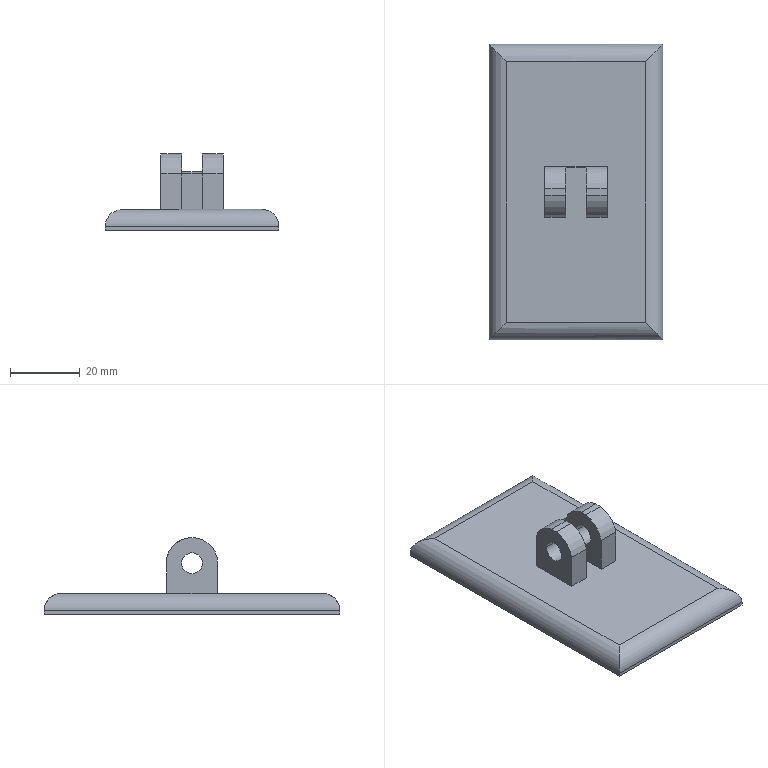Part | SolidWorks | features ICE 3, Extrusion 1, Fillet 1 | 1 solid | 27 faces | box 50 x 85 x 22 mm | volume 26297 mm3 | plane 16 | cylinder 11 | commonest cylinder face diameters 6 x4 10 x4 14.776 x3
STEP:
#1=CARTESIAN_POINT('',(34.,45.508,14.673));
#2=VERTEX_POINT('',#1);
#3=CARTESIAN_POINT('',(34.,39.508,14.673));
#4=VERTEX_POINT('',#3);
#5=CARTESIAN_POINT('',(34.,42.508,14.673));
#6=DIRECTION('',(-1.,0.,0.));
#7=DIRECTION('',(0.,-1.,0.));
#8=AXIS2_PLACEMENT_3D('',#5,#6,#7);
#9=CIRCLE('',#8,3.);
#10=EDGE_CURVE('',#2,#4,#9,.T.);
#11=ORIENTED_EDGE('',*,*,#10,.F.);
#12=CARTESIAN_POINT('',(28.,45.508,14.673));
#13=VERTEX_POINT('',#12);
#14=CARTESIAN_POINT('',(50.,45.508,14.673));
#15=DIRECTION('',(-1.,0.,0.));
#16=VECTOR('',#15,1000.);
#17=LINE('',#14,#16);
#18=EDGE_CURVE('',#2,#13,#17,.T.);
#19=ORIENTED_EDGE('',*,*,#18,.T.);
#20=CARTESIAN_POINT('',(28.,39.508,14.673));
#21=VERTEX_POINT('',#20);
#22=CARTESIAN_POINT('',(28.,42.508,14.673));
#23=DIRECTION('',(1.,0.,0.));
#24=DIRECTION('',(0.,1.,0.));
#25=AXIS2_PLACEMENT_3D('',#22,#23,#24);
#26=CIRCLE('',#25,3.);
#27=EDGE_CURVE('',#21,#13,#26,.T.);
#28=ORIENTED_EDGE('',*,*,#27,.F.);
#29=CARTESIAN_POINT('',(50.,39.508,14.673));
#30=DIRECTION('',(-1.,0.,0.));
#31=VECTOR('',#30,1000.);
#32=LINE('',#29,#31);
#33=EDGE_CURVE('',#4,#21,#32,.T.);
#34=ORIENTED_EDGE('',*,*,#33,.F.);
#35=EDGE_LOOP('',(#11,#19,#28,#34));
#36=FACE_OUTER_BOUND('',#35,.T.);
#37=CARTESIAN_POINT('',(50.,42.508,14.673));
#38=DIRECTION('',(-1.,0.,0.));
#39=DIRECTION('',(0.,-1.,0.));
#40=AXIS2_PLACEMENT_3D('',#37,#38,#39);
#41=CYLINDRICAL_SURFACE('',#40,3.);
#42=ADVANCED_FACE('',(#36),#41,.F.);
#43=CARTESIAN_POINT('',(22.,45.508,14.673));
#44=VERTEX_POINT('',#43);
#45=CARTESIAN_POINT('',(22.,39.508,14.673));
#46=VERTEX_POINT('',#45);
#47=CARTESIAN_POINT('',(22.,42.508,14.673));
#48=DIRECTION('',(-1.,0.,0.));
#49=DIRECTION('',(0.,-1.,0.));
#50=AXIS2_PLACEMENT_3D('',#47,#48,#49);
#51=CIRCLE('',#50,3.);
#52=EDGE_CURVE('',#44,#46,#51,.T.);
#53=ORIENTED_EDGE('',*,*,#52,.F.);
#54=CARTESIAN_POINT('',(16.,45.508,14.673));
#55=VERTEX_POINT('',#54);
#56=CARTESIAN_POINT('',(50.,45.508,14.673));
#57=DIRECTION('',(-1.,0.,0.));
#58=VECTOR('',#57,1000.);
#59=LINE('',#56,#58);
#60=EDGE_CURVE('',#44,#55,#59,.T.);
#61=ORIENTED_EDGE('',*,*,#60,.T.);
#62=CARTESIAN_POINT('',(16.,39.508,14.673));
#63=VERTEX_POINT('',#62);
#64=CARTESIAN_POINT('',(16.,42.508,14.673));
#65=DIRECTION('',(-1.,0.,0.));
#66=DIRECTION('',(0.,-1.,0.));
#67=AXIS2_PLACEMENT_3D('',#64,#65,#66);
#68=CIRCLE('',#67,3.);
#69=EDGE_CURVE('',#55,#63,#68,.T.);
#70=ORIENTED_EDGE('',*,*,#69,.T.);
#71=CARTESIAN_POINT('',(50.,39.508,14.673));
#72=DIRECTION('',(-1.,0.,0.));
#73=VECTOR('',#72,1000.);
#74=LINE('',#71,#73);
#75=EDGE_CURVE('',#46,#63,#74,.T.);
#76=ORIENTED_EDGE('',*,*,#75,.F.);
#77=EDGE_LOOP('',(#53,#61,#70,#76));
#78=FACE_OUTER_BOUND('',#77,.T.);
#79=CARTESIAN_POINT('',(50.,42.508,14.673));
#80=DIRECTION('',(-1.,0.,0.));
#81=DIRECTION('',(0.,-1.,0.));
#82=AXIS2_PLACEMENT_3D('',#79,#80,#81);
#83=CYLINDRICAL_SURFACE('',#82,3.);
#84=ADVANCED_FACE('',(#78),#83,.F.);
#85=CARTESIAN_POINT('',(16.,43.457,22.));
#86=VERTEX_POINT('',#85);
#87=CARTESIAN_POINT('',(22.,43.457,22.));
#88=VERTEX_POINT('',#87);
#89=CARTESIAN_POINT('',(50.,43.457,22.));
#90=DIRECTION('',(1.,0.,0.));
#91=VECTOR('',#90,1000.);
#92=LINE('',#89,#91);
#93=EDGE_CURVE('',#86,#88,#92,.T.);
#94=ORIENTED_EDGE('',*,*,#93,.F.);
#95=CARTESIAN_POINT('',(16.,41.559,22.));
#96=VERTEX_POINT('',#95);
#97=CARTESIAN_POINT('',(16.,49.724,22.));
#98=DIRECTION('',(0.,-1.,0.));
#99=VECTOR('',#98,1000.);
#100=LINE('',#97,#99);
#101=EDGE_CURVE('',#86,#96,#100,.T.);
#102=ORIENTED_EDGE('',*,*,#101,.T.);
#103=CARTESIAN_POINT('',(22.,41.559,22.));
#104=VERTEX_POINT('',#103);
#105=CARTESIAN_POINT('',(50.,41.559,22.));
#106=DIRECTION('',(-1.,0.,0.));
#107=VECTOR('',#106,1000.);
#108=LINE('',#105,#107);
#109=EDGE_CURVE('',#104,#96,#108,.T.);
#110=ORIENTED_EDGE('',*,*,#109,.F.);
#111=CARTESIAN_POINT('',(22.,49.57,22.));
#112=DIRECTION('',(0.,-1.,0.));
#113=VECTOR('',#112,1000.);
#114=LINE('',#111,#113);
#115=EDGE_CURVE('',#88,#104,#114,.T.);
#116=ORIENTED_EDGE('',*,*,#115,.F.);
#117=EDGE_LOOP('',(#94,#102,#110,#116));
#118=FACE_OUTER_BOUND('',#117,.T.);
#119=CARTESIAN_POINT('',(0.,0.,22.));
#120=DIRECTION('',(0.,0.,1.));
#121=DIRECTION('',(1.,0.,0.));
#122=AXIS2_PLACEMENT_3D('',#119,#120,#121);
#123=PLANE('',#122);
#124=ADVANCED_FACE('',(#118),#123,.T.);
#125=CARTESIAN_POINT('',(34.,35.276,16.183));
#126=VERTEX_POINT('',#125);
#127=CARTESIAN_POINT('',(34.,35.276,6.));
#128=VERTEX_POINT('',#127);
#129=CARTESIAN_POINT('',(34.,35.276,22.));
#130=DIRECTION('',(0.,0.,-1.));
#131=VECTOR('',#130,1000.);
#132=LINE('',#129,#131);
#133=EDGE_CURVE('',#126,#128,#132,.T.);
#134=ORIENTED_EDGE('',*,*,#133,.F.);
#135=CARTESIAN_POINT('',(28.,35.276,16.183));
#136=VERTEX_POINT('',#135);
#137=CARTESIAN_POINT('',(50.,35.276,16.183));
#138=DIRECTION('',(-1.,0.,0.));
#139=VECTOR('',#138,1000.);
#140=LINE('',#137,#139);
#141=EDGE_CURVE('',#126,#136,#140,.T.);
#142=ORIENTED_EDGE('',*,*,#141,.T.);
#143=CARTESIAN_POINT('',(28.,35.276,6.));
#144=VERTEX_POINT('',#143);
#145=CARTESIAN_POINT('',(28.,35.276,22.));
#146=DIRECTION('',(0.,0.,-1.));
#147=VECTOR('',#146,1000.);
#148=LINE('',#145,#147);
#149=EDGE_CURVE('',#136,#144,#148,.T.);
#150=ORIENTED_EDGE('',*,*,#149,.T.);
#151=CARTESIAN_POINT('',(16.,35.276,6.));
#152=DIRECTION('',(1.,0.,0.));
#153=VECTOR('',#152,1000.);
#154=LINE('',#151,#153);
#155=EDGE_CURVE('',#144,#128,#154,.T.);
#156=ORIENTED_EDGE('',*,*,#155,.T.);
#157=EDGE_LOOP('',(#134,#142,#150,#156));
#158=FACE_OUTER_BOUND('',#157,.T.);
#159=CARTESIAN_POINT('',(16.,35.276,22.));
#160=DIRECTION('',(0.,1.,0.));
#161=DIRECTION('',(0.,0.,1.));
#162=AXIS2_PLACEMENT_3D('',#159,#160,#161);
#163=PLANE('',#162);
#164=ADVANCED_FACE('',(#158),#163,.F.);
#165=CARTESIAN_POINT('',(5.,80.,6.));
#166=VERTEX_POINT('',#165);
#167=CARTESIAN_POINT('',(5.,5.,6.));
#168=VERTEX_POINT('',#167);
#169=CARTESIAN_POINT('',(5.,0.,6.));
#170=DIRECTION('',(0.,-1.,0.));
#171=VECTOR('',#170,1000.);
#172=LINE('',#169,#171);
#173=EDGE_CURVE('',#166,#168,#172,.T.);
#174=ORIENTED_EDGE('',*,*,#173,.T.);
#175=CARTESIAN_POINT('',(45.,5.,6.));
#176=VERTEX_POINT('',#175);
#177=CARTESIAN_POINT('',(0.,5.,6.));
#178=DIRECTION('',(1.,0.,0.));
#179=VECTOR('',#178,1000.);
#180=LINE('',#177,#179);
#181=EDGE_CURVE('',#168,#176,#180,.T.);
#182=ORIENTED_EDGE('',*,*,#181,.T.);
#183=CARTESIAN_POINT('',(45.,80.,6.));
#184=VERTEX_POINT('',#183);
#185=CARTESIAN_POINT('',(45.,0.,6.));
#186=DIRECTION('',(0.,1.,0.));
#187=VECTOR('',#186,1000.);
#188=LINE('',#185,#187);
#189=EDGE_CURVE('',#176,#184,#188,.T.);
#190=ORIENTED_EDGE('',*,*,#189,.T.);
#191=CARTESIAN_POINT('',(0.,80.,6.));
#192=DIRECTION('',(-1.,0.,0.));
#193=VECTOR('',#192,1000.);
#194=LINE('',#191,#193);
#195=EDGE_CURVE('',#184,#166,#194,.T.);
#196=ORIENTED_EDGE('',*,*,#195,.T.);
#197=EDGE_LOOP('',(#174,#182,#190,#196));
#198=FACE_OUTER_BOUND('',#197,.T.);
#199=ORIENTED_EDGE('',*,*,#155,.F.);
#200=CARTESIAN_POINT('',(28.,49.57,6.));
#201=VERTEX_POINT('',#200);
#202=CARTESIAN_POINT('',(28.,49.57,6.));
#203=DIRECTION('',(0.,1.,0.));
#204=VECTOR('',#203,1000.);
#205=LINE('',#202,#204);
#206=EDGE_CURVE('',#144,#201,#205,.T.);
#207=ORIENTED_EDGE('',*,*,#206,.T.);
#208=CARTESIAN_POINT('',(22.,49.57,6.));
#209=VERTEX_POINT('',#208);
#210=CARTESIAN_POINT('',(22.,49.57,6.));
#211=DIRECTION('',(-1.,0.,0.));
#212=VECTOR('',#211,1000.);
#213=LINE('',#210,#212);
#214=EDGE_CURVE('',#201,#209,#213,.T.);
#215=ORIENTED_EDGE('',*,*,#214,.T.);
#216=CARTESIAN_POINT('',(22.,35.276,6.));
#217=VERTEX_POINT('',#216);
#218=CARTESIAN_POINT('',(22.,49.57,6.));
#219=DIRECTION('',(0.,-1.,0.));
#220=VECTOR('',#219,1000.);
#221=LINE('',#218,#220);
#222=EDGE_CURVE('',#209,#217,#221,.T.);
#223=ORIENTED_EDGE('',*,*,#222,.T.);
#224=CARTESIAN_POINT('',(16.,35.276,6.));
#225=VERTEX_POINT('',#224);
#226=CARTESIAN_POINT('',(16.,35.276,6.));
#227=DIRECTION('',(1.,0.,0.));
#228=VECTOR('',#227,1000.);
#229=LINE('',#226,#228);
#230=EDGE_CURVE('',#225,#217,#229,.T.);
#231=ORIENTED_EDGE('',*,*,#230,.F.);
#232=CARTESIAN_POINT('',(16.,49.724,6.));
#233=VERTEX_POINT('',#232);
#234=CARTESIAN_POINT('',(16.,49.724,6.));
#235=DIRECTION('',(0.,-1.,0.));
#236=VECTOR('',#235,1000.);
#237=LINE('',#234,#236);
#238=EDGE_CURVE('',#233,#225,#237,.T.);
#239=ORIENTED_EDGE('',*,*,#238,.F.);
#240=CARTESIAN_POINT('',(34.,49.724,6.));
#241=VERTEX_POINT('',#240);
#242=CARTESIAN_POINT('',(16.,49.724,6.));
#243=DIRECTION('',(-1.,0.,0.));
#244=VECTOR('',#243,1000.);
#245=LINE('',#242,#244);
#246=EDGE_CURVE('',#241,#233,#245,.T.);
#247=ORIENTED_EDGE('',*,*,#246,.F.);
#248=CARTESIAN_POINT('',(34.,49.724,6.));
#249=DIRECTION('',(0.,1.,0.));
#250=VECTOR('',#249,1000.);
#251=LINE('',#248,#250);
#252=EDGE_CURVE('',#128,#241,#251,.T.);
#253=ORIENTED_EDGE('',*,*,#252,.F.);
#254=EDGE_LOOP('',(#199,#207,#215,#223,#231,#239,#247,#253));
#255=FACE_BOUND('',#254,.T.);
#256=CARTESIAN_POINT('',(0.,0.,6.));
#257=DIRECTION('',(0.,0.,-1.));
#258=DIRECTION('',(-1.,0.,0.));
#259=AXIS2_PLACEMENT_3D('',#256,#257,#258);
#260=PLANE('',#259);
#261=ADVANCED_FACE('',(#198,#255),#260,.F.);
#262=CARTESIAN_POINT('',(0.,0.,1.));
#263=VERTEX_POINT('',#262);
#264=CARTESIAN_POINT('',(0.,0.,0.));
#265=VERTEX_POINT('',#264);
#266=CARTESIAN_POINT('',(0.,0.,6.));
#267=DIRECTION('',(0.,0.,-1.));
#268=VECTOR('',#267,1000.);
#269=LINE('',#266,#268);
#270=EDGE_CURVE('',#263,#265,#269,.T.);
#271=ORIENTED_EDGE('',*,*,#270,.F.);
#272=CARTESIAN_POINT('',(0.,85.,1.));
#273=VERTEX_POINT('',#272);
#274=CARTESIAN_POINT('',(0.,0.,1.));
#275=DIRECTION('',(0.,1.,0.));
#276=VECTOR('',#275,1000.);
#277=LINE('',#274,#276);
#278=EDGE_CURVE('',#263,#273,#277,.T.);
#279=ORIENTED_EDGE('',*,*,#278,.T.);
#280=CARTESIAN_POINT('',(0.,85.,0.));
#281=VERTEX_POINT('',#280);
#282=CARTESIAN_POINT('',(0.,85.,6.));
#283=DIRECTION('',(0.,0.,-1.));
#284=VECTOR('',#283,1000.);
#285=LINE('',#282,#284);
#286=EDGE_CURVE('',#273,#281,#285,.T.);
#287=ORIENTED_EDGE('',*,*,#286,.T.);
#288=CARTESIAN_POINT('',(0.,0.,0.));
#289=DIRECTION('',(0.,-1.,0.));
#290=VECTOR('',#289,1000.);
#291=LINE('',#288,#290);
#292=EDGE_CURVE('',#281,#265,#291,.T.);
#293=ORIENTED_EDGE('',*,*,#292,.T.);
#294=EDGE_LOOP('',(#271,#279,#287,#293));
#295=FACE_OUTER_BOUND('',#294,.T.);
#296=CARTESIAN_POINT('',(0.,0.,6.));
#297=DIRECTION('',(1.,0.,0.));
#298=DIRECTION('',(0.,0.,-1.));
#299=AXIS2_PLACEMENT_3D('',#296,#297,#298);
#300=PLANE('',#299);
#301=ADVANCED_FACE('',(#295),#300,.F.);
#302=CARTESIAN_POINT('',(50.,0.,1.));
#303=VERTEX_POINT('',#302);
#304=CARTESIAN_POINT('',(50.,0.,0.));
#305=VERTEX_POINT('',#304);
#306=CARTESIAN_POINT('',(50.,0.,6.));
#307=DIRECTION('',(0.,0.,-1.));
#308=VECTOR('',#307,1000.);
#309=LINE('',#306,#308);
#310=EDGE_CURVE('',#303,#305,#309,.T.);
#311=ORIENTED_EDGE('',*,*,#310,.F.);
#312=CARTESIAN_POINT('',(0.,0.,1.));
#313=DIRECTION('',(-1.,0.,0.));
#314=VECTOR('',#313,1000.);
#315=LINE('',#312,#314);
#316=EDGE_CURVE('',#303,#263,#315,.T.);
#317=ORIENTED_EDGE('',*,*,#316,.T.);
#318=ORIENTED_EDGE('',*,*,#270,.T.);
#319=CARTESIAN_POINT('',(0.,0.,0.));
#320=DIRECTION('',(1.,0.,0.));
#321=VECTOR('',#320,1000.);
#322=LINE('',#319,#321);
#323=EDGE_CURVE('',#265,#305,#322,.T.);
#324=ORIENTED_EDGE('',*,*,#323,.T.);
#325=EDGE_LOOP('',(#311,#317,#318,#324));
#326=FACE_OUTER_BOUND('',#325,.T.);
#327=CARTESIAN_POINT('',(0.,0.,6.));
#328=DIRECTION('',(0.,1.,0.));
#329=DIRECTION('',(0.,0.,1.));
#330=AXIS2_PLACEMENT_3D('',#327,#328,#329);
#331=PLANE('',#330);
#332=ADVANCED_FACE('',(#326),#331,.F.);
#333=CARTESIAN_POINT('',(50.,85.,1.));
#334=VERTEX_POINT('',#333);
#335=CARTESIAN_POINT('',(50.,85.,0.));
#336=VERTEX_POINT('',#335);
#337=CARTESIAN_POINT('',(50.,85.,6.));
#338=DIRECTION('',(0.,0.,-1.));
#339=VECTOR('',#338,1000.);
#340=LINE('',#337,#339);
#341=EDGE_CURVE('',#334,#336,#340,.T.);
#342=ORIENTED_EDGE('',*,*,#341,.F.);
#343=CARTESIAN_POINT('',(50.,0.,1.));
#344=DIRECTION('',(0.,-1.,0.));
#345=VECTOR('',#344,1000.);
#346=LINE('',#343,#345);
#347=EDGE_CURVE('',#334,#303,#346,.T.);
#348=ORIENTED_EDGE('',*,*,#347,.T.);
#349=ORIENTED_EDGE('',*,*,#310,.T.);
#350=CARTESIAN_POINT('',(50.,0.,0.));
#351=DIRECTION('',(0.,1.,0.));
#352=VECTOR('',#351,1000.);
#353=LINE('',#350,#352);
#354=EDGE_CURVE('',#305,#336,#353,.T.);
#355=ORIENTED_EDGE('',*,*,#354,.T.);
#356=EDGE_LOOP('',(#342,#348,#349,#355));
#357=FACE_OUTER_BOUND('',#356,.T.);
#358=CARTESIAN_POINT('',(50.,0.,6.));
#359=DIRECTION('',(-1.,0.,0.));
#360=DIRECTION('',(0.,0.,1.));
#361=AXIS2_PLACEMENT_3D('',#358,#359,#360);
#362=PLANE('',#361);
#363=ADVANCED_FACE('',(#357),#362,.F.);
#364=ORIENTED_EDGE('',*,*,#286,.F.);
#365=CARTESIAN_POINT('',(0.,85.,1.));
#366=DIRECTION('',(1.,0.,0.));
#367=VECTOR('',#366,1000.);
#368=LINE('',#365,#367);
#369=EDGE_CURVE('',#273,#334,#368,.T.);
#370=ORIENTED_EDGE('',*,*,#369,.T.);
#371=ORIENTED_EDGE('',*,*,#341,.T.);
#372=CARTESIAN_POINT('',(0.,85.,0.));
#373=DIRECTION('',(-1.,0.,0.));
#374=VECTOR('',#373,1000.);
#375=LINE('',#372,#374);
#376=EDGE_CURVE('',#336,#281,#375,.T.);
#377=ORIENTED_EDGE('',*,*,#376,.T.);
#378=EDGE_LOOP('',(#364,#370,#371,#377));
#379=FACE_OUTER_BOUND('',#378,.T.);
#380=CARTESIAN_POINT('',(0.,85.,6.));
#381=DIRECTION('',(0.,-1.,0.));
#382=DIRECTION('',(0.,0.,-1.));
#383=AXIS2_PLACEMENT_3D('',#380,#381,#382);
#384=PLANE('',#383);
#385=ADVANCED_FACE('',(#379),#384,.F.);
#386=ORIENTED_EDGE('',*,*,#292,.F.);
#387=ORIENTED_EDGE('',*,*,#376,.F.);
#388=ORIENTED_EDGE('',*,*,#354,.F.);
#389=ORIENTED_EDGE('',*,*,#323,.F.);
#390=EDGE_LOOP('',(#386,#387,#388,#389));
#391=FACE_OUTER_BOUND('',#390,.T.);
#392=CARTESIAN_POINT('',(0.,0.,0.));
#393=DIRECTION('',(0.,0.,-1.));
#394=DIRECTION('',(-1.,0.,0.));
#395=AXIS2_PLACEMENT_3D('',#392,#393,#394);
#396=PLANE('',#395);
#397=ADVANCED_FACE('',(#391),#396,.T.);
#398=CARTESIAN_POINT('',(34.,42.508,14.673));
#399=DIRECTION('',(-1.,0.,0.));
#400=DIRECTION('',(0.,-1.,0.));
#401=AXIS2_PLACEMENT_3D('',#398,#399,#400);
#402=CIRCLE('',#401,3.);
#403=EDGE_CURVE('',#4,#2,#402,.T.);
#404=ORIENTED_EDGE('',*,*,#403,.T.);
#405=ORIENTED_EDGE('',*,*,#10,.T.);
#406=EDGE_LOOP('',(#404,#405));
#407=FACE_BOUND('',#406,.T.);
#408=CARTESIAN_POINT('',(34.,49.724,16.256));
#409=VERTEX_POINT('',#408);
#410=CARTESIAN_POINT('',(34.,49.724,22.));
#411=DIRECTION('',(0.,0.,-1.));
#412=VECTOR('',#411,1000.);
#413=LINE('',#410,#412);
#414=EDGE_CURVE('',#409,#241,#413,.T.);
#415=ORIENTED_EDGE('',*,*,#414,.F.);
#416=CARTESIAN_POINT('',(34.,43.457,22.));
#417=VERTEX_POINT('',#416);
#418=CARTESIAN_POINT('',(34.,42.508,14.673));
#419=DIRECTION('',(1.,0.,0.));
#420=DIRECTION('',(0.,-1.,0.));
#421=AXIS2_PLACEMENT_3D('',#418,#419,#420);
#422=CIRCLE('',#421,7.388);
#423=EDGE_CURVE('',#409,#417,#422,.T.);
#424=ORIENTED_EDGE('',*,*,#423,.T.);
#425=CARTESIAN_POINT('',(34.,41.559,22.));
#426=VERTEX_POINT('',#425);
#427=CARTESIAN_POINT('',(34.,49.724,22.));
#428=DIRECTION('',(0.,1.,0.));
#429=VECTOR('',#428,1000.);
#430=LINE('',#427,#429);
#431=EDGE_CURVE('',#426,#417,#430,.T.);
#432=ORIENTED_EDGE('',*,*,#431,.F.);
#433=CARTESIAN_POINT('',(34.,42.508,14.673));
#434=DIRECTION('',(1.,0.,0.));
#435=DIRECTION('',(0.,-1.,0.));
#436=AXIS2_PLACEMENT_3D('',#433,#434,#435);
#437=CIRCLE('',#436,7.388);
#438=EDGE_CURVE('',#426,#126,#437,.T.);
#439=ORIENTED_EDGE('',*,*,#438,.T.);
#440=ORIENTED_EDGE('',*,*,#133,.T.);
#441=ORIENTED_EDGE('',*,*,#252,.T.);
#442=EDGE_LOOP('',(#415,#424,#432,#439,#440,#441));
#443=FACE_OUTER_BOUND('',#442,.T.);
#444=CARTESIAN_POINT('',(34.,49.724,22.));
#445=DIRECTION('',(-1.,0.,0.));
#446=DIRECTION('',(0.,-1.,0.));
#447=AXIS2_PLACEMENT_3D('',#444,#445,#446);
#448=PLANE('',#447);
#449=ADVANCED_FACE('',(#407,#443),#448,.F.);
#450=CARTESIAN_POINT('',(16.,49.724,16.256));
#451=VERTEX_POINT('',#450);
#452=CARTESIAN_POINT('',(16.,49.724,22.));
#453=DIRECTION('',(0.,0.,-1.));
#454=VECTOR('',#453,1000.);
#455=LINE('',#452,#454);
#456=EDGE_CURVE('',#451,#233,#455,.T.);
#457=ORIENTED_EDGE('',*,*,#456,.F.);
#458=CARTESIAN_POINT('',(50.,49.724,16.256));
#459=DIRECTION('',(1.,0.,0.));
#460=VECTOR('',#459,1000.);
#461=LINE('',#458,#460);
#462=EDGE_CURVE('',#451,#409,#461,.T.);
#463=ORIENTED_EDGE('',*,*,#462,.T.);
#464=ORIENTED_EDGE('',*,*,#414,.T.);
#465=ORIENTED_EDGE('',*,*,#246,.T.);
#466=EDGE_LOOP('',(#457,#463,#464,#465));
#467=FACE_OUTER_BOUND('',#466,.T.);
#468=CARTESIAN_POINT('',(16.,49.724,22.));
#469=DIRECTION('',(0.,-1.,0.));
#470=DIRECTION('',(0.,0.,-1.));
#471=AXIS2_PLACEMENT_3D('',#468,#469,#470);
#472=PLANE('',#471);
#473=ADVANCED_FACE('',(#467),#472,.F.);
#474=CARTESIAN_POINT('',(16.,42.508,14.673));
#475=DIRECTION('',(-1.,0.,0.));
#476=DIRECTION('',(0.,-1.,0.));
#477=AXIS2_PLACEMENT_3D('',#474,#475,#476);
#478=CIRCLE('',#477,3.);
#479=EDGE_CURVE('',#63,#55,#478,.T.);
#480=ORIENTED_EDGE('',*,*,#479,.F.);
#481=ORIENTED_EDGE('',*,*,#69,.F.);
#482=EDGE_LOOP('',(#480,#481));
#483=FACE_BOUND('',#482,.T.);
#484=CARTESIAN_POINT('',(16.,35.276,16.183));
#485=VERTEX_POINT('',#484);
#486=CARTESIAN_POINT('',(16.,35.276,22.));
#487=DIRECTION('',(0.,0.,-1.));
#488=VECTOR('',#487,1000.);
#489=LINE('',#486,#488);
#490=EDGE_CURVE('',#485,#225,#489,.T.);
#491=ORIENTED_EDGE('',*,*,#490,.F.);
#492=CARTESIAN_POINT('',(16.,42.508,14.673));
#493=DIRECTION('',(1.,0.,0.));
#494=DIRECTION('',(0.,-1.,0.));
#495=AXIS2_PLACEMENT_3D('',#492,#493,#494);
#496=CIRCLE('',#495,7.388);
#497=EDGE_CURVE('',#96,#485,#496,.T.);
#498=ORIENTED_EDGE('',*,*,#497,.F.);
#499=ORIENTED_EDGE('',*,*,#101,.F.);
#500=CARTESIAN_POINT('',(16.,42.508,14.673));
#501=DIRECTION('',(1.,0.,0.));
#502=DIRECTION('',(0.,-1.,0.));
#503=AXIS2_PLACEMENT_3D('',#500,#501,#502);
#504=CIRCLE('',#503,7.388);
#505=EDGE_CURVE('',#451,#86,#504,.T.);
#506=ORIENTED_EDGE('',*,*,#505,.F.);
#507=ORIENTED_EDGE('',*,*,#456,.T.);
#508=ORIENTED_EDGE('',*,*,#238,.T.);
#509=EDGE_LOOP('',(#491,#498,#499,#506,#507,#508));
#510=FACE_OUTER_BOUND('',#509,.T.);
#511=CARTESIAN_POINT('',(16.,49.724,22.));
#512=DIRECTION('',(1.,0.,0.));
#513=DIRECTION('',(0.,0.,-1.));
#514=AXIS2_PLACEMENT_3D('',#511,#512,#513);
#515=PLANE('',#514);
#516=ADVANCED_FACE('',(#483,#510),#515,.F.);
#517=CARTESIAN_POINT('',(22.,35.276,16.183));
#518=VERTEX_POINT('',#517);
#519=CARTESIAN_POINT('',(22.,35.276,22.));
#520=DIRECTION('',(0.,0.,1.));
#521=VECTOR('',#520,1000.);
#522=LINE('',#519,#521);
#523=EDGE_CURVE('',#217,#518,#522,.T.);
#524=ORIENTED_EDGE('',*,*,#523,.T.);
#525=CARTESIAN_POINT('',(50.,35.276,16.183));
#526=DIRECTION('',(-1.,0.,0.));
#527=VECTOR('',#526,1000.);
#528=LINE('',#525,#527);
#529=EDGE_CURVE('',#518,#485,#528,.T.);
#530=ORIENTED_EDGE('',*,*,#529,.T.);
#531=ORIENTED_EDGE('',*,*,#490,.T.);
#532=ORIENTED_EDGE('',*,*,#230,.T.);
#533=EDGE_LOOP('',(#524,#530,#531,#532));
#534=FACE_OUTER_BOUND('',#533,.T.);
#535=CARTESIAN_POINT('',(16.,35.276,22.));
#536=DIRECTION('',(0.,1.,0.));
#537=DIRECTION('',(0.,0.,1.));
#538=AXIS2_PLACEMENT_3D('',#535,#536,#537);
#539=PLANE('',#538);
#540=ADVANCED_FACE('',(#534),#539,.F.);
#541=CARTESIAN_POINT('',(28.,43.457,22.));
#542=VERTEX_POINT('',#541);
#543=CARTESIAN_POINT('',(50.,43.457,22.));
#544=DIRECTION('',(1.,0.,0.));
#545=VECTOR('',#544,1000.);
#546=LINE('',#543,#545);
#547=EDGE_CURVE('',#542,#417,#546,.T.);
#548=ORIENTED_EDGE('',*,*,#547,.F.);
#549=CARTESIAN_POINT('',(28.,41.559,22.));
#550=VERTEX_POINT('',#549);
#551=CARTESIAN_POINT('',(28.,0.,22.));
#552=DIRECTION('',(0.,1.,0.));
#553=VECTOR('',#552,1000.);
#554=LINE('',#551,#553);
#555=EDGE_CURVE('',#550,#542,#554,.T.);
#556=ORIENTED_EDGE('',*,*,#555,.F.);
#557=CARTESIAN_POINT('',(50.,41.559,22.));
#558=DIRECTION('',(-1.,0.,0.));
#559=VECTOR('',#558,1000.);
#560=LINE('',#557,#559);
#561=EDGE_CURVE('',#426,#550,#560,.T.);
#562=ORIENTED_EDGE('',*,*,#561,.F.);
#563=ORIENTED_EDGE('',*,*,#431,.T.);
#564=EDGE_LOOP('',(#548,#556,#562,#563));
#565=FACE_OUTER_BOUND('',#564,.T.);
#566=CARTESIAN_POINT('',(0.,0.,22.));
#567=DIRECTION('',(0.,0.,1.));
#568=DIRECTION('',(1.,0.,0.));
#569=AXIS2_PLACEMENT_3D('',#566,#567,#568);
#570=PLANE('',#569);
#571=ADVANCED_FACE('',(#565),#570,.T.);
#572=CARTESIAN_POINT('',(50.,85.,1.));
#573=CARTESIAN_POINT('',(50.,85.,3.929));
#574=CARTESIAN_POINT('',(47.929,82.929,6.));
#575=CARTESIAN_POINT('',(45.,80.,6.));
#576=(BOUNDED_CURVE()B_SPLINE_CURVE(3,(#572,#573,#574,#575),.UNSPECIFIED.,.F.,.T.)B_SPLINE_CURVE_WITH_KNOTS((4,4),(3.142,4.712),.UNSPECIFIED.)CURVE()GEOMETRIC_REPRESENTATION_ITEM()RATIONAL_B_SPLINE_CURVE((1.,0.8047,0.8047,1.))REPRESENTATION_ITEM(''));
#577=EDGE_CURVE('',#334,#184,#576,.T.);
#578=ORIENTED_EDGE('',*,*,#577,.F.);
#579=ORIENTED_EDGE('',*,*,#369,.F.);
#580=CARTESIAN_POINT('',(5.,80.,6.));
#581=CARTESIAN_POINT('',(2.071,82.929,6.));
#582=CARTESIAN_POINT('',(0.,85.,3.929));
#583=CARTESIAN_POINT('',(0.,85.,1.));
#584=(BOUNDED_CURVE()B_SPLINE_CURVE(3,(#580,#581,#582,#583),.UNSPECIFIED.,.F.,.F.)B_SPLINE_CURVE_WITH_KNOTS((4,4),(1.571,3.142),.UNSPECIFIED.)CURVE()GEOMETRIC_REPRESENTATION_ITEM()RATIONAL_B_SPLINE_CURVE((1.,0.8047,0.8047,1.))REPRESENTATION_ITEM(''));
#585=EDGE_CURVE('',#166,#273,#584,.T.);
#586=ORIENTED_EDGE('',*,*,#585,.F.);
#587=ORIENTED_EDGE('',*,*,#195,.F.);
#588=EDGE_LOOP('',(#578,#579,#586,#587));
#589=FACE_OUTER_BOUND('',#588,.T.);
#590=CARTESIAN_POINT('',(0.,80.,1.));
#591=DIRECTION('',(-1.,0.,0.));
#592=DIRECTION('',(0.,0.,1.));
#593=AXIS2_PLACEMENT_3D('',#590,#591,#592);
#594=CYLINDRICAL_SURFACE('',#593,5.);
#595=ADVANCED_FACE('',(#589),#594,.T.);
#596=ORIENTED_EDGE('',*,*,#585,.T.);
#597=ORIENTED_EDGE('',*,*,#278,.F.);
#598=CARTESIAN_POINT('',(5.,5.,6.));
#599=CARTESIAN_POINT('',(2.071,2.071,6.));
#600=CARTESIAN_POINT('',(0.,0.,3.929));
#601=CARTESIAN_POINT('',(0.,0.,1.));
#602=(BOUNDED_CURVE()B_SPLINE_CURVE(3,(#598,#599,#600,#601),.UNSPECIFIED.,.F.,.T.)B_SPLINE_CURVE_WITH_KNOTS((4,4),(4.712,6.283),.UNSPECIFIED.)CURVE()GEOMETRIC_REPRESENTATION_ITEM()RATIONAL_B_SPLINE_CURVE((1.,0.8047,0.8047,1.))REPRESENTATION_ITEM(''));
#603=EDGE_CURVE('',#168,#263,#602,.T.);
#604=ORIENTED_EDGE('',*,*,#603,.F.);
#605=ORIENTED_EDGE('',*,*,#173,.F.);
#606=EDGE_LOOP('',(#596,#597,#604,#605));
#607=FACE_OUTER_BOUND('',#606,.T.);
#608=CARTESIAN_POINT('',(5.,0.,1.));
#609=DIRECTION('',(0.,-1.,0.));
#610=DIRECTION('',(0.,0.,-1.));
#611=AXIS2_PLACEMENT_3D('',#608,#609,#610);
#612=CYLINDRICAL_SURFACE('',#611,5.);
#613=ADVANCED_FACE('',(#607),#612,.T.);
#614=ORIENTED_EDGE('',*,*,#577,.T.);
#615=ORIENTED_EDGE('',*,*,#189,.F.);
#616=CARTESIAN_POINT('',(50.,0.,1.));
#617=CARTESIAN_POINT('',(50.,0.,3.929));
#618=CARTESIAN_POINT('',(47.929,2.071,6.));
#619=CARTESIAN_POINT('',(45.,5.,6.));
#620=(BOUNDED_CURVE()B_SPLINE_CURVE(3,(#616,#617,#618,#619),.UNSPECIFIED.,.F.,.T.)B_SPLINE_CURVE_WITH_KNOTS((4,4),(3.142,4.712),.UNSPECIFIED.)CURVE()GEOMETRIC_REPRESENTATION_ITEM()RATIONAL_B_SPLINE_CURVE((1.,0.8047,0.8047,1.))REPRESENTATION_ITEM(''));
#621=EDGE_CURVE('',#303,#176,#620,.T.);
#622=ORIENTED_EDGE('',*,*,#621,.F.);
#623=ORIENTED_EDGE('',*,*,#347,.F.);
#624=EDGE_LOOP('',(#614,#615,#622,#623));
#625=FACE_OUTER_BOUND('',#624,.T.);
#626=CARTESIAN_POINT('',(45.,0.,1.));
#627=DIRECTION('',(0.,1.,0.));
#628=DIRECTION('',(0.,0.,1.));
#629=AXIS2_PLACEMENT_3D('',#626,#627,#628);
#630=CYLINDRICAL_SURFACE('',#629,5.);
#631=ADVANCED_FACE('',(#625),#630,.T.);
#632=ORIENTED_EDGE('',*,*,#603,.T.);
#633=ORIENTED_EDGE('',*,*,#316,.F.);
#634=ORIENTED_EDGE('',*,*,#621,.T.);
#635=ORIENTED_EDGE('',*,*,#181,.F.);
#636=EDGE_LOOP('',(#632,#633,#634,#635));
#637=FACE_OUTER_BOUND('',#636,.T.);
#638=CARTESIAN_POINT('',(0.,5.,1.));
#639=DIRECTION('',(1.,0.,0.));
#640=DIRECTION('',(0.,0.,-1.));
#641=AXIS2_PLACEMENT_3D('',#638,#639,#640);
#642=CYLINDRICAL_SURFACE('',#641,5.);
#643=ADVANCED_FACE('',(#637),#642,.T.);
#644=ORIENTED_EDGE('',*,*,#27,.T.);
#645=CARTESIAN_POINT('',(28.,42.508,14.673));
#646=DIRECTION('',(1.,0.,0.));
#647=DIRECTION('',(0.,1.,0.));
#648=AXIS2_PLACEMENT_3D('',#645,#646,#647);
#649=CIRCLE('',#648,3.);
#650=EDGE_CURVE('',#13,#21,#649,.T.);
#651=ORIENTED_EDGE('',*,*,#650,.T.);
#652=EDGE_LOOP('',(#644,#651));
#653=FACE_BOUND('',#652,.T.);
#654=ORIENTED_EDGE('',*,*,#149,.F.);
#655=CARTESIAN_POINT('',(28.,42.508,14.673));
#656=DIRECTION('',(-1.,0.,0.));
#657=DIRECTION('',(0.,1.,0.));
#658=AXIS2_PLACEMENT_3D('',#655,#656,#657);
#659=CIRCLE('',#658,7.388);
#660=EDGE_CURVE('',#136,#550,#659,.T.);
#661=ORIENTED_EDGE('',*,*,#660,.T.);
#662=ORIENTED_EDGE('',*,*,#555,.T.);
#663=CARTESIAN_POINT('',(28.,49.57,16.842));
#664=VERTEX_POINT('',#663);
#665=CARTESIAN_POINT('',(28.,42.508,14.673));
#666=DIRECTION('',(-1.,0.,0.));
#667=DIRECTION('',(0.,1.,0.));
#668=AXIS2_PLACEMENT_3D('',#665,#666,#667);
#669=CIRCLE('',#668,7.388);
#670=EDGE_CURVE('',#542,#664,#669,.T.);
#671=ORIENTED_EDGE('',*,*,#670,.T.);
#672=CARTESIAN_POINT('',(28.,49.57,6.));
#673=DIRECTION('',(0.,0.,1.));
#674=VECTOR('',#673,1000.);
#675=LINE('',#672,#674);
#676=EDGE_CURVE('',#201,#664,#675,.T.);
#677=ORIENTED_EDGE('',*,*,#676,.F.);
#678=ORIENTED_EDGE('',*,*,#206,.F.);
#679=EDGE_LOOP('',(#654,#661,#662,#671,#677,#678));
#680=FACE_OUTER_BOUND('',#679,.T.);
#681=CARTESIAN_POINT('',(28.,49.57,6.));
#682=DIRECTION('',(1.,0.,0.));
#683=DIRECTION('',(0.,1.,0.));
#684=AXIS2_PLACEMENT_3D('',#681,#682,#683);
#685=PLANE('',#684);
#686=ADVANCED_FACE('',(#653,#680),#685,.F.);
#687=CARTESIAN_POINT('',(22.,42.508,14.673));
#688=DIRECTION('',(-1.,0.,0.));
#689=DIRECTION('',(0.,-1.,0.));
#690=AXIS2_PLACEMENT_3D('',#687,#688,#689);
#691=CIRCLE('',#690,3.);
#692=EDGE_CURVE('',#46,#44,#691,.T.);
#693=ORIENTED_EDGE('',*,*,#692,.T.);
#694=ORIENTED_EDGE('',*,*,#52,.T.);
#695=EDGE_LOOP('',(#693,#694));
#696=FACE_BOUND('',#695,.T.);
#697=CARTESIAN_POINT('',(22.,49.57,16.842));
#698=VERTEX_POINT('',#697);
#699=CARTESIAN_POINT('',(22.,49.57,6.));
#700=DIRECTION('',(0.,0.,1.));
#701=VECTOR('',#700,1000.);
#702=LINE('',#699,#701);
#703=EDGE_CURVE('',#209,#698,#702,.T.);
#704=ORIENTED_EDGE('',*,*,#703,.T.);
#705=CARTESIAN_POINT('',(22.,42.508,14.673));
#706=DIRECTION('',(1.,0.,0.));
#707=DIRECTION('',(0.,-1.,0.));
#708=AXIS2_PLACEMENT_3D('',#705,#706,#707);
#709=CIRCLE('',#708,7.388);
#710=EDGE_CURVE('',#698,#88,#709,.T.);
#711=ORIENTED_EDGE('',*,*,#710,.T.);
#712=ORIENTED_EDGE('',*,*,#115,.T.);
#713=CARTESIAN_POINT('',(22.,42.508,14.673));
#714=DIRECTION('',(1.,0.,0.));
#715=DIRECTION('',(0.,-1.,0.));
#716=AXIS2_PLACEMENT_3D('',#713,#714,#715);
#717=CIRCLE('',#716,7.388);
#718=EDGE_CURVE('',#104,#518,#717,.T.);
#719=ORIENTED_EDGE('',*,*,#718,.T.);
#720=ORIENTED_EDGE('',*,*,#523,.F.);
#721=ORIENTED_EDGE('',*,*,#222,.F.);
#722=EDGE_LOOP('',(#704,#711,#712,#719,#720,#721));
#723=FACE_OUTER_BOUND('',#722,.T.);
#724=CARTESIAN_POINT('',(22.,49.57,6.));
#725=DIRECTION('',(-1.,0.,0.));
#726=DIRECTION('',(0.,-1.,0.));
#727=AXIS2_PLACEMENT_3D('',#724,#725,#726);
#728=PLANE('',#727);
#729=ADVANCED_FACE('',(#696,#723),#728,.F.);
#730=ORIENTED_EDGE('',*,*,#676,.T.);
#731=CARTESIAN_POINT('',(50.,49.57,16.842));
#732=DIRECTION('',(-1.,0.,0.));
#733=VECTOR('',#732,1000.);
#734=LINE('',#731,#733);
#735=EDGE_CURVE('',#664,#698,#734,.T.);
#736=ORIENTED_EDGE('',*,*,#735,.T.);
#737=ORIENTED_EDGE('',*,*,#703,.F.);
#738=ORIENTED_EDGE('',*,*,#214,.F.);
#739=EDGE_LOOP('',(#730,#736,#737,#738));
#740=FACE_OUTER_BOUND('',#739,.T.);
#741=CARTESIAN_POINT('',(22.,49.57,6.));
#742=DIRECTION('',(0.,1.,0.));
#743=DIRECTION('',(0.,0.,1.));
#744=AXIS2_PLACEMENT_3D('',#741,#742,#743);
#745=PLANE('',#744);
#746=ADVANCED_FACE('',(#740),#745,.F.);
#747=ORIENTED_EDGE('',*,*,#505,.T.);
#748=ORIENTED_EDGE('',*,*,#93,.T.);
#749=ORIENTED_EDGE('',*,*,#710,.F.);
#750=ORIENTED_EDGE('',*,*,#735,.F.);
#751=ORIENTED_EDGE('',*,*,#670,.F.);
#752=ORIENTED_EDGE('',*,*,#547,.T.);
#753=ORIENTED_EDGE('',*,*,#423,.F.);
#754=ORIENTED_EDGE('',*,*,#462,.F.);
#755=EDGE_LOOP('',(#747,#748,#749,#750,#751,#752,#753,#754));
#756=FACE_OUTER_BOUND('',#755,.T.);
#757=CARTESIAN_POINT('',(50.,42.508,14.673));
#758=DIRECTION('',(-1.,0.,0.));
#759=DIRECTION('',(0.,-1.,0.));
#760=AXIS2_PLACEMENT_3D('',#757,#758,#759);
#761=CYLINDRICAL_SURFACE('',#760,7.388);
#762=ADVANCED_FACE('',(#756),#761,.T.);
#763=ORIENTED_EDGE('',*,*,#60,.F.);
#764=ORIENTED_EDGE('',*,*,#692,.F.);
#765=ORIENTED_EDGE('',*,*,#75,.T.);
#766=ORIENTED_EDGE('',*,*,#479,.T.);
#767=EDGE_LOOP('',(#763,#764,#765,#766));
#768=FACE_OUTER_BOUND('',#767,.T.);
#769=CARTESIAN_POINT('',(50.,42.508,14.673));
#770=DIRECTION('',(-1.,0.,0.));
#771=DIRECTION('',(0.,-1.,0.));
#772=AXIS2_PLACEMENT_3D('',#769,#770,#771);
#773=CYLINDRICAL_SURFACE('',#772,3.);
#774=ADVANCED_FACE('',(#768),#773,.F.);
#775=ORIENTED_EDGE('',*,*,#718,.F.);
#776=ORIENTED_EDGE('',*,*,#109,.T.);
#777=ORIENTED_EDGE('',*,*,#497,.T.);
#778=ORIENTED_EDGE('',*,*,#529,.F.);
#779=EDGE_LOOP('',(#775,#776,#777,#778));
#780=FACE_OUTER_BOUND('',#779,.T.);
#781=CARTESIAN_POINT('',(50.,42.508,14.673));
#782=DIRECTION('',(-1.,0.,0.));
#783=DIRECTION('',(0.,-1.,0.));
#784=AXIS2_PLACEMENT_3D('',#781,#782,#783);
#785=CYLINDRICAL_SURFACE('',#784,7.388);
#786=ADVANCED_FACE('',(#780),#785,.T.);
#787=ORIENTED_EDGE('',*,*,#18,.F.);
#788=ORIENTED_EDGE('',*,*,#403,.F.);
#789=ORIENTED_EDGE('',*,*,#33,.T.);
#790=ORIENTED_EDGE('',*,*,#650,.F.);
#791=EDGE_LOOP('',(#787,#788,#789,#790));
#792=FACE_OUTER_BOUND('',#791,.T.);
#793=CARTESIAN_POINT('',(50.,42.508,14.673));
#794=DIRECTION('',(-1.,0.,0.));
#795=DIRECTION('',(0.,-1.,0.));
#796=AXIS2_PLACEMENT_3D('',#793,#794,#795);
#797=CYLINDRICAL_SURFACE('',#796,3.);
#798=ADVANCED_FACE('',(#792),#797,.F.);
#799=ORIENTED_EDGE('',*,*,#438,.F.);
#800=ORIENTED_EDGE('',*,*,#561,.T.);
#801=ORIENTED_EDGE('',*,*,#660,.F.);
#802=ORIENTED_EDGE('',*,*,#141,.F.);
#803=EDGE_LOOP('',(#799,#800,#801,#802));
#804=FACE_OUTER_BOUND('',#803,.T.);
#805=CARTESIAN_POINT('',(50.,42.508,14.673));
#806=DIRECTION('',(-1.,0.,0.));
#807=DIRECTION('',(0.,-1.,0.));
#808=AXIS2_PLACEMENT_3D('',#805,#806,#807);
#809=CYLINDRICAL_SURFACE('',#808,7.388);
#810=ADVANCED_FACE('',(#804),#809,.T.);
#811=CLOSED_SHELL('',(#42,#84,#124,#164,#261,#301,#332,#363,#385,#397,#449,#473,#516,#540,#571,#595,#613,#631,#643,#686,#729,#746,#762,#774,#786,#798,#810));
#812=MANIFOLD_SOLID_BREP('',#811);
#813=CARTESIAN_POINT('',(0.,0.,0.));
#814=DIRECTION('',(0.,0.,1.));
#815=DIRECTION('',(1.,0.,0.));
#816=AXIS2_PLACEMENT_3D('',#813,#814,#815);
#817=(LENGTH_UNIT()NAMED_UNIT(*)SI_UNIT(.MILLI.,.METRE.));
#818=UNCERTAINTY_MEASURE_WITH_UNIT(LENGTH_MEASURE(0.00001),#817,'','');
#819=(NAMED_UNIT(*)PLANE_ANGLE_UNIT()SI_UNIT($,.RADIAN.));
#820=(NAMED_UNIT(*)SI_UNIT($,.STERADIAN.)SOLID_ANGLE_UNIT());
#821=(GEOMETRIC_REPRESENTATION_CONTEXT(3)GLOBAL_UNCERTAINTY_ASSIGNED_CONTEXT((#818))GLOBAL_UNIT_ASSIGNED_CONTEXT((#817,#819,#820))REPRESENTATION_CONTEXT('',''));
#822=ADVANCED_BREP_SHAPE_REPRESENTATION('',(#812,#816),#821);